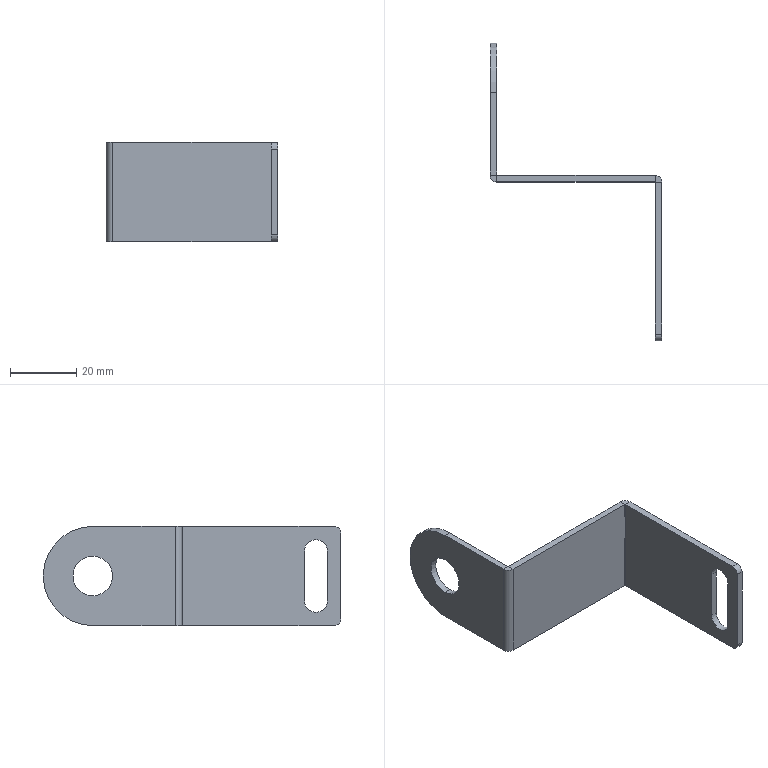Part | STEP file | Proximity switch bracket 2 | 1 solid | 31 faces | box 52 x 90 x 30 mm | volume 7634 mm3 | plane 19 | cylinder 12 | commonest cylinder face diameters 0.2 x2 4 x2 4.2 x2 7 x2 12 x2 30 x2